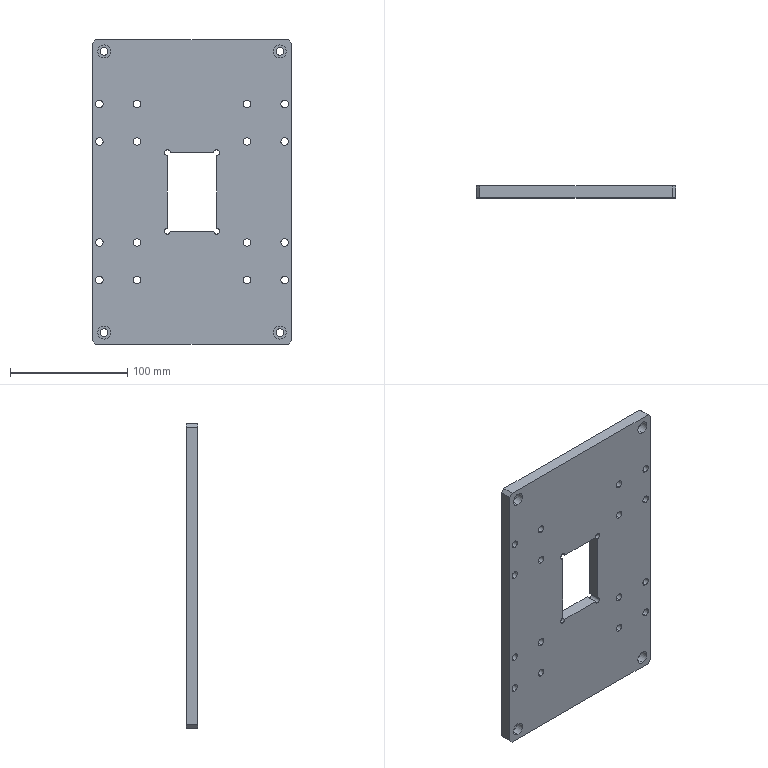Part | STEP file | 0-19 Mounting plate 1 | 1 solid | 72 faces | box 170 x 10 x 260 mm | volume 404759 mm3 | cylinder 54 | plane 18 | commonest cylinder face diameters 6.5 x32 6.6 x8 11 x8 5 x6